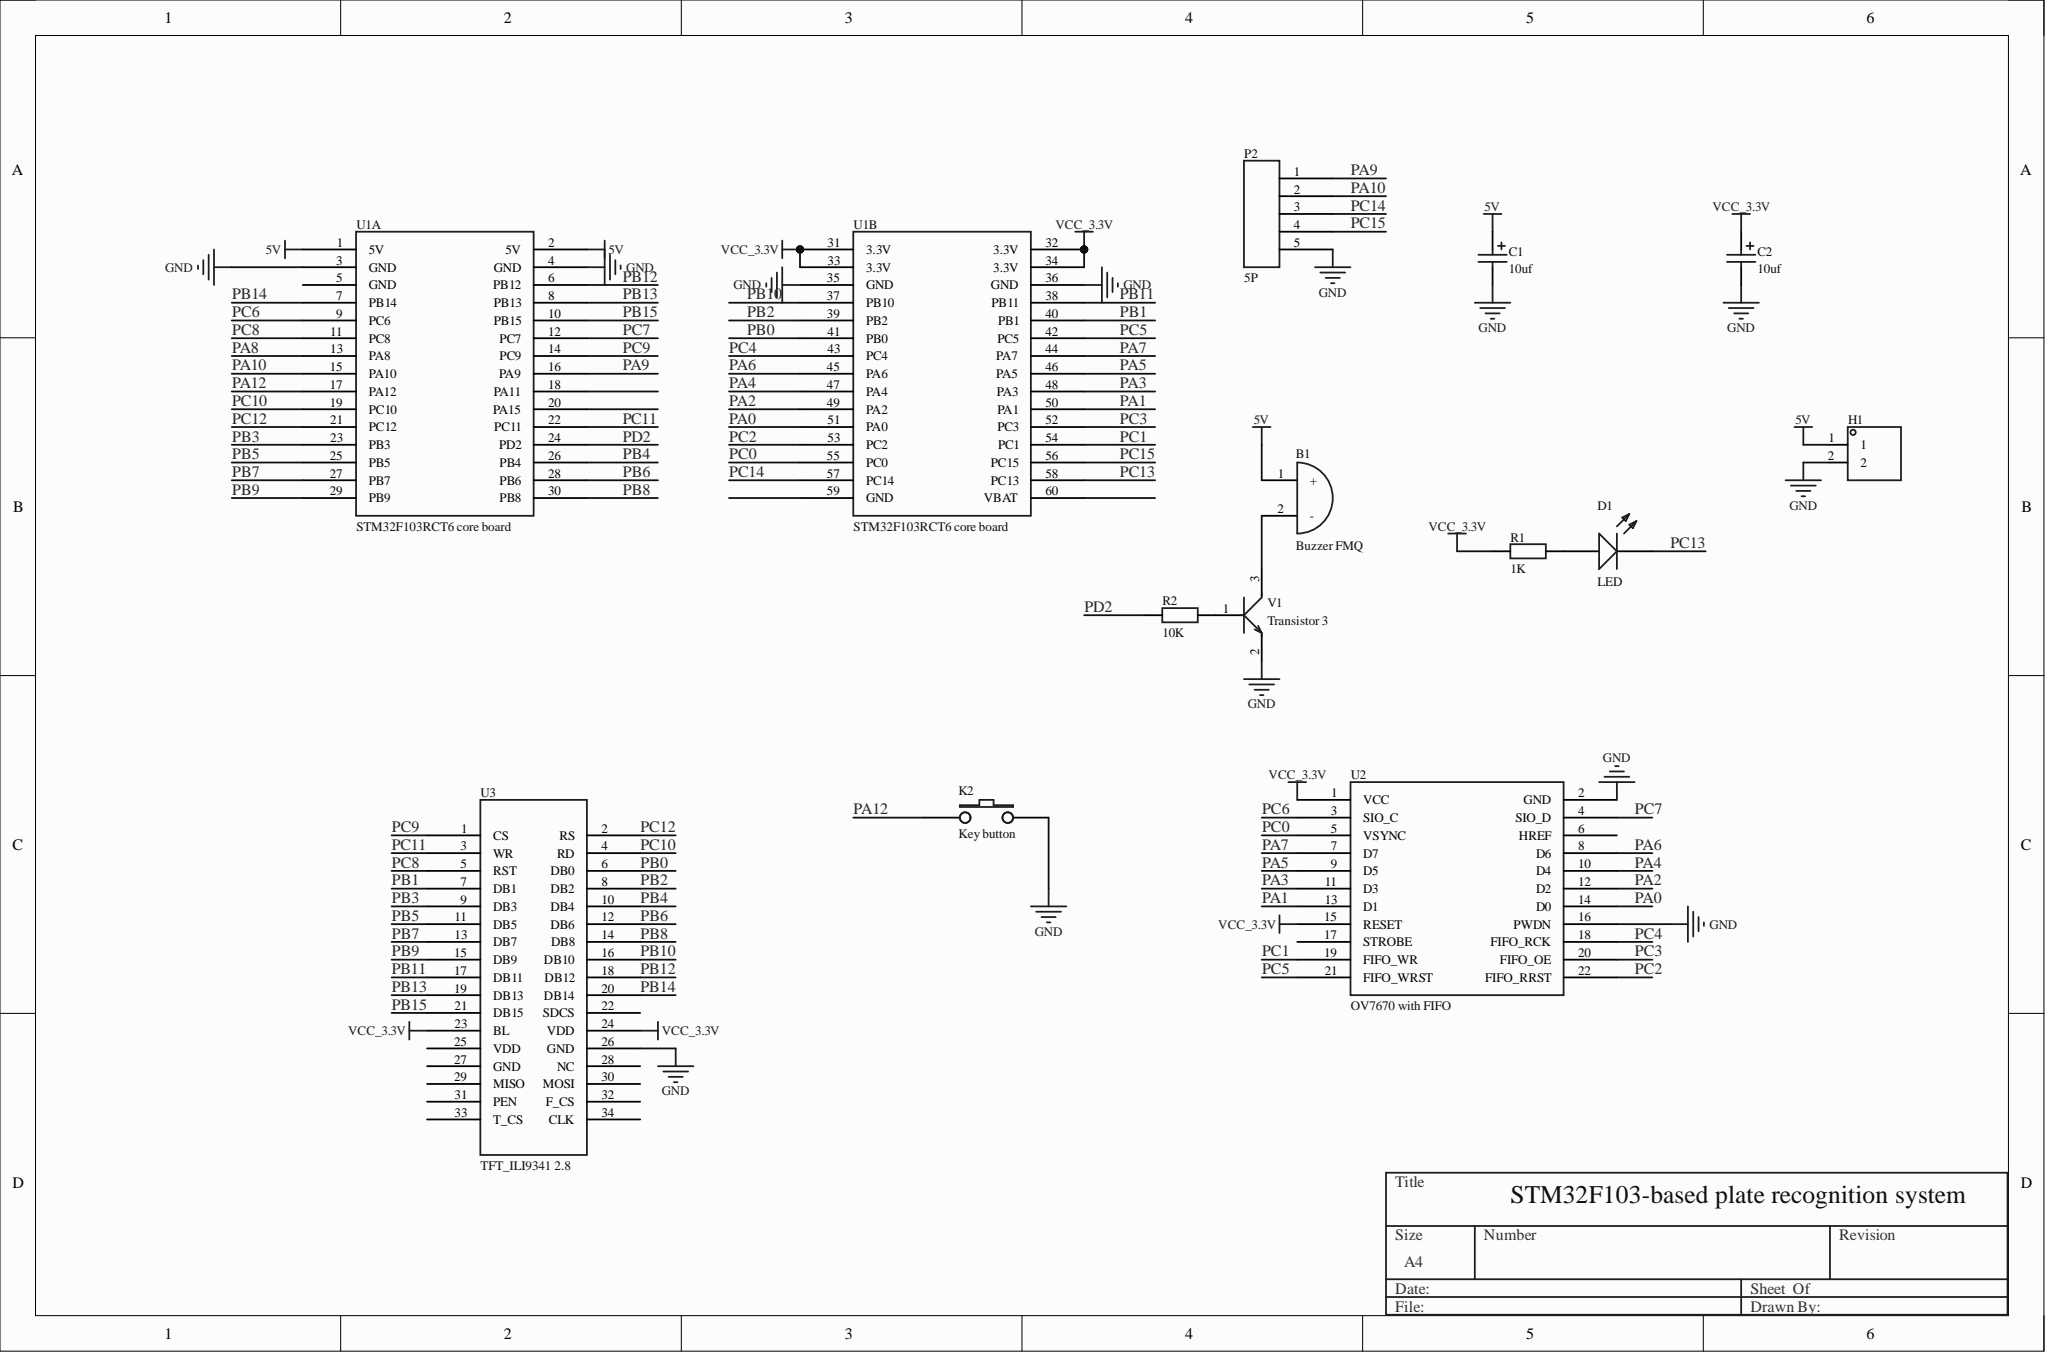Circuit board | Altium Designer | 13 parts | 50 nets
Bill of materials:
Comment,Description,Designator,Footprint,LibRef,Quantity
"Buzzer FMQ","","B1","蜂鸣器","蜂鸣器FMQ","1"
"10uf","","C1, C2","CD0.254cm","10uf","2"
"LED","","D1","发光二极管FZ","发光二级管","1"
"","","H1","HDR-TH_2P-P2.54-V-M-1","HDR-M_2.54_1x2P","1"
"Key button","","K2","按键","key按键","1"
"5P","","P2","5ZHEN-100mil","5P","1"
"1K","","R1","电阻FZ","1K","1"
"10K","","R2","电阻FZ","10K","1"
"STM32F103RCT6 core board","","U1","STM32F103RC/RB 核心板","STM32F103RCT6核心板","1"
"OV7670 with FIFO","FIFO","U2","OV7670模块","OV7670 with FIFO","1"
"TFT_ILI9341 2.8","ILI9341","U3","2.8寸TFT","TFT_ILI9341 2.8","1"
"Transistor 3","","V1","三极管FZ","三极管3","1"
Netlist (Protel format):
[
B1
蜂鸣器
Buzzer FMQ



]
[
C1
CD0.254cm
10uf



]
[
C2
CD0.254cm
10uf



]
[
D1
发光二极管FZ
LED



]
[
H1
HDR-TH_2P-P2.54-V-M-1




]
[
K2
按键
Key button



]
[
P2
5ZHEN-100mil
5P



]
[
R1
电阻FZ
1K



]
[
R2
电阻FZ
10K



]
[
U1
STM32F103RC/RB 核心板
STM32F103RCT6 core board



]
[
U2
OV7670模块
OV7670 with FIFO



]
[
U3
2.8寸TFT
TFT_ILI9341 2.8



]
[
V1
三极管FZ
Transistor 3



]
(
VCC_3.3V
C2-1
R1-1
U1-31
U1-32
U1-33
U1-34
U2-1
U2-15
U3-23
U3-24
)
(
PD2
R2-1
U1-24
)
(
PC15
P2-4
U1-56
)
(
PC14
P2-3
U1-57
)
(
PC13
D1-2
U1-58
)
(
PC12
U1-21
U3-2
)
(
PC11
U1-22
U3-3
)
(
PC10
U1-19
U3-4
)
(
PC9
U1-14
U3-1
)
(
PC8
U1-11
U3-5
)
(
PC7
U1-12
U2-4
)
(
PC6
U1-9
U2-3
)
(
PC5
U1-42
U2-21
)
(
PC4
U1-43
U2-18
)
(
PC3
U1-52
U2-20
)
(
PC2
U1-53
U2-22
)
(
PC1
U1-54
U2-19
)
(
PC0
U1-55
U2-5
)
(
PB15
U1-10
U3-21
)
(
PB14
U1-7
U3-20
)
(
PB13
U1-8
U3-19
)
(
PB12
U1-6
U3-18
)
(
PB11
U1-38
U3-17
)
(
PB10
U1-37
U3-16
)
(
PB9
U1-29
U3-15
)
(
PB8
U1-30
U3-14
)
(
PB7
U1-27
U3-13
)
(
PB6
U1-28
U3-12
)
(
PB5
U1-25
U3-11
)
(
PB4
U1-26
U3-10
)
(
PB3
U1-23
U3-9
)
(
PB2
U1-39
U3-8
)
(
PB1
U1-40
U3-7
)
(
PB0
U1-41
U3-6
)
(
PA12
K2-1
U1-17
)
(
PA10
P2-2
U1-15
)
(
PA9
P2-1
U1-16
)
(
PA7
U1-44
U2-7
)
(
PA6
U1-45
U2-8
)
(
PA5
U1-46
U2-9
)
(
PA4
U1-47
U2-10
)
(
PA3
U1-48
U2-11
)
(
PA2
U1-49
U2-12
)
(
PA1
U1-50
U2-13
)
(
PA0
U1-51
U2-14
)
(
NetR2_2
R2-2
V1-1
)
(
NetD1_1
D1-1
R1-2
)
(
NetB1_2
B1-2
V1-3
)
(
GND
C1-2
C2-2
H1-2
K2-2
P2-5
U1-3
U1-4
U1-35
U1-36
U2-2
U2-16
U3-26
V1-2
)
(
5V
B1-1
C1-1
H1-1
U1-1
U1-2
)